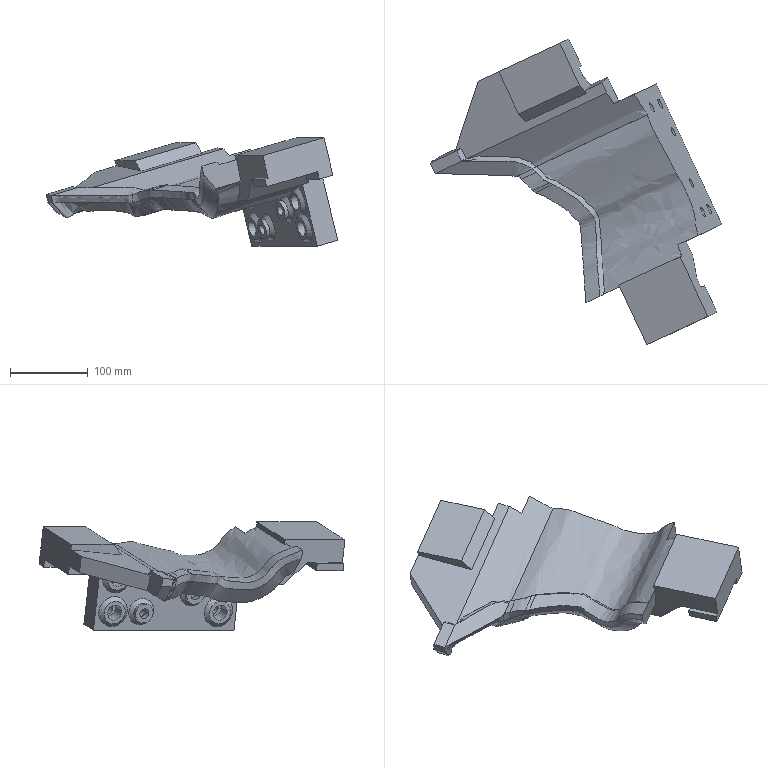Part | NX | features solid 2 | 1 solid | 97 faces | box 376.203 x 394.526 x 140.059 mm | volume 2389400 mm3 | plane 62 | spline 15 | cylinder 14 | cone 6 | commonest cylinder face diameters 13 x6 20 x4 12 x2 25 x2